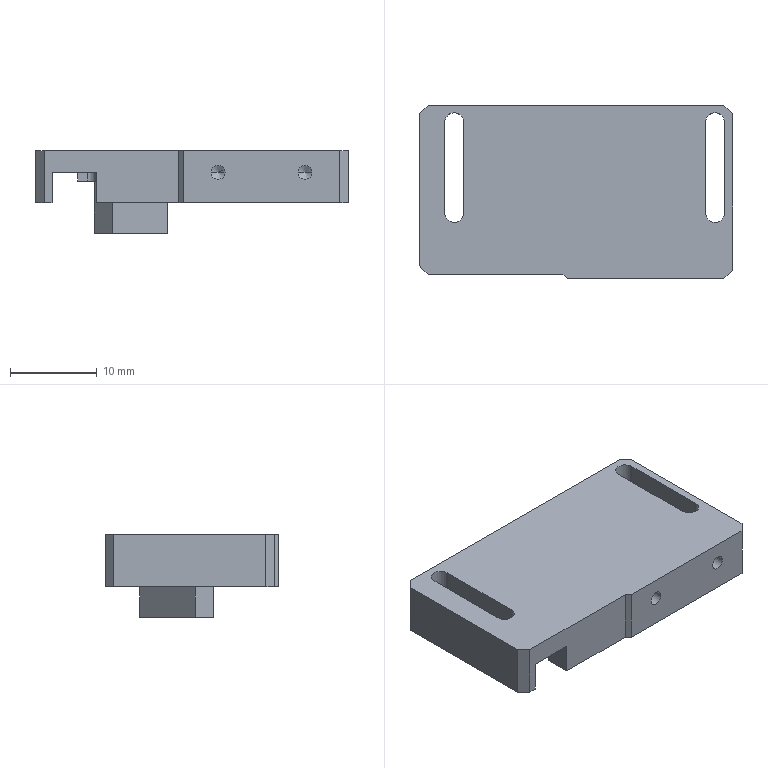NC program | NX | posted with a generic post | part box 36 x 20 x 9.5 mm
Lines 4413 to 4561 of 4561:
(ZLEVEL_PROFILE_1 , TOOL : D6A45)
N8788 T07 M6
N8790 G54
N8792 G17 G0 G90 X-5.627 Y-8.018 S9500 M3
N8794 G43 Z30. H7
N8796 Z1.
N8798 G94 G1 Z-1. F1250.
N8800 X-5.42 Y-7.245
N8802 G3 X-5.575 Y-6.665 R0.6
N8804 G1 X-11.943 Y-0.297
N8806 G2 X-11.943 Y1.054 R0.956
N8808 G1 X-9.818 Y3.18
N8810 G2 X-8.466 Y3.18 R0.956
N8812 G1 X-2.098 Y-3.188
N8814 G2 X-2.098 Y-4.54 R0.956
N8816 G1 X-4.224 Y-6.665
N8818 G2 X-5.575 Y-6.665 R0.956
N8820 G3 X-6.155 Y-6.51 R0.6
N8822 G1 X-7.159 Y-6.779
N8824 Z1.
N8826 G0 Z30.
(ZLEVEL_PROFILE_1_COPY , TOOL : D6A45)
N8828 X-12.497 Y4.943
N8830 Z-2.5
N8832 G1 Z-4.5
N8834 X-10.668 Y5.391
N8836 G3 X-10.928 Y5.541 R0.3
N8838 G1 X-11.003
N8840 G2 X-11.959 Y6.497 R0.956
N8842 G1 Y9.503
N8844 G2 X-11.003 Y10.459 R0.956
N8846 G1 X-1.897
N8848 X-1.676 Y10.68
N8850 G2 X-1.003 Y10.959 R0.952
N8852 G1 X17.003
N8854 G2 X17.676 Y10.68 R0.952
N8856 G1 X18.68 Y9.676
N8858 G2 X18.959 Y9.003 R0.952
N8860 G1 Y6.497
N8862 G2 X18.003 Y5.541 R0.956
N8864 G1 X-7.371
N8866 G3 X-7.63 Y5.391 R0.3
N8868 G1 X-5.185 Y4.341
N8870 Z-2.5
N8872 G0 Z30.
N8874 X-14.148 Y10.423
N8876 Z-2.5
N8878 G1 Z-4.5
N8880 X-14.841 Y10.023
N8882 G3 X-15.141 Y9.503 R0.6
N8884 G1 Y-10.003
N8886 G2 X-16.097 Y-10.959 R0.956
N8888 G1 X-17.003
N8890 G2 X-17.676 Y-10.68 R0.952
N8892 G1 X-18.68 Y-9.676
N8894 G2 X-18.959 Y-9.003 R0.952
N8896 G1 Y8.503
N8898 G2 X-18.68 Y9.176 R0.952
N8900 G1 X-17.676 Y10.18
N8902 G2 X-17.01 Y10.459 R0.944
N8904 G1 X-16.097
N8906 G2 X-15.141 Y9.503 R0.956
N8908 G3 X-14.841 Y8.983 R0.6
N8910 G1 X-13.941 Y8.464
N8912 Z-2.5
N8914 G0 Z30.
N8916 X16.001 Y4.341
N8918 Z-2.5
N8920 G1 Z-4.5
N8922 X15.159 Y4.366
N8924 G3 X14.859 Y3.846 R0.6
N8926 G1 Y-10.003
N8928 G2 X13.903 Y-10.959 R0.979
N8930 G1 X10.897
N8932 G2 X9.941 Y-10.003 R0.956
N8934 G1 Y0.857
N8936 G2 X10.22 Y1.519 R0.939
N8938 G1 X13.224 Y4.524
N8940 G2 X14.859 Y3.846 R0.957
N8942 G3 X15.158 Y3.326 R0.6
N8944 G1 X16.059 Y2.807
N8946 Z-2.5
N8948 G0 Z30.
(ZLEVEL_PROFILE_1_COPY_COPY , TOOL : D6A45)
N8950 X7.414 Y-12.159
N8952 Z-6.
N8954 G1 Z-8.
N8956 X7.777 Y-11.109
N8958 G3 X7.517 Y-10.959 R0.3
N8960 G1 X-12.704
N8962 G3 X-12.963 Y-11.109 R0.3
N8964 G1 X-12.614 Y-12.159
N8966 Z-6.
N8968 G0 Z30.
N8970 X20.159 Y3.014
N8972 Z-6.
N8974 G1 Z-8.
N8976 X19.109 Y3.379
N8978 G3 X18.959 Y3.12 R0.3
N8980 G1 Y-9.003
N8982 G2 X18.68 Y-9.676 R0.952
N8984 G1 X17.676 Y-10.68
N8986 X17.289 Y-10.907
N8988 G3 X16.993 Y-11.429 R0.6
N8990 G1 X17.002 Y-12.681
N8992 Z-6.
N8994 G0 Z30.
N8996 M5
(111 , TOOL : D6)
N8998 T06 M6
N9000 G54
N9002 G17 G0 G90 X18.388 Y-14.804 S9500 M3
N9004 G43 Z30. H6
N9006 Z-7.35
N9008 G94 G1 Z-9.35 F1000.
N9010 X17.52 Y-13.3
N9012 G3 X17. Y-13. R0.6
N9014 G1 X-17. F1200.
N9016 G2 X-19.121 Y-12.121 R3.
N9018 G1 X-20.121 Y-11.121
N9020 G2 X-21. Y-9. R3.
N9022 G1 Y8.5
N9024 G2 X-20.121 Y10.621 R3.
N9026 G1 X-19.121 Y11.621
N9028 G2 X-17. Y12.5 R3.
N9030 G1 X-2.658
N9032 G2 X-1. Y13. R3.
N9034 G1 X17.
N9036 G2 X19.121 Y12.121 R3.
N9038 G1 X20.121 Y11.121
N9040 G2 X21. Y9. R3.
N9042 G1 Y-9.
N9044 G2 X20.121 Y-11.121 R3.
N9046 G1 X19.121 Y-12.121
N9048 G2 X17. Y-13. R3.
N9050 G3 X16.48 Y-13.3 R0.6
N9052 G1 X15.499 Y-15.
N9054 Z-7.35
N9056 G0 Z30.
N9058 M5
N9060 M2